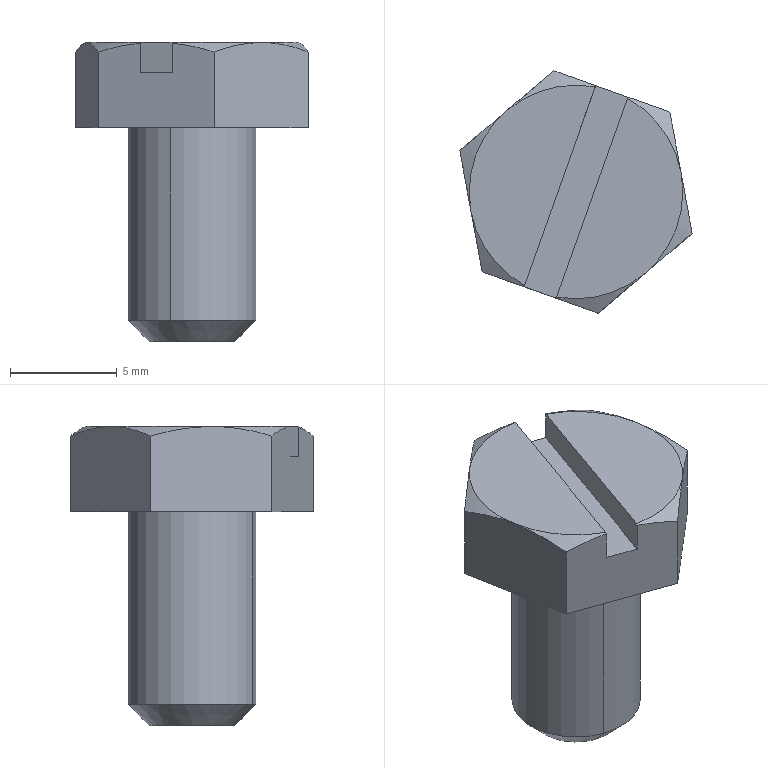Part | SolidWorks | features BaseBody 1 | 1 solid | 23 faces | box 10.878 x 11.357 x 14 mm | volume 597.287 mm3 | plane 13 | cone 8 | cylinder 2 | commonest cylinder face diameters 6 x2
STEP:
#1=CARTESIAN_POINT('',(398.719,157.843,50.8));
#2=VERTEX_POINT('',#1);
#3=CARTESIAN_POINT('',(400.061,161.611,50.8));
#4=VERTEX_POINT('',#3);
#5=CARTESIAN_POINT('',(399.39,159.727,50.8));
#6=DIRECTION('',(0.,0.,-1.));
#7=DIRECTION('',(-0.3355,-0.942,0.));
#8=AXIS2_PLACEMENT_3D('',#5,#6,#7);
#9=CIRCLE('',#8,2.);
#10=EDGE_CURVE('',#2,#4,#9,.T.);
#11=ORIENTED_EDGE('',*,*,#10,.F.);
#12=CARTESIAN_POINT('',(398.384,156.9,51.8));
#13=VERTEX_POINT('',#12);
#14=CARTESIAN_POINT('',(398.719,157.843,50.8));
#15=DIRECTION('',(-0.2372,-0.6661,0.7071));
#16=VECTOR('',#15,1000.);
#17=LINE('',#14,#16);
#18=EDGE_CURVE('',#2,#13,#17,.T.);
#19=ORIENTED_EDGE('',*,*,#18,.T.);
#20=CARTESIAN_POINT('',(400.396,162.553,51.8));
#21=VERTEX_POINT('',#20);
#22=CARTESIAN_POINT('',(399.39,159.727,51.8));
#23=DIRECTION('',(0.,0.,1.));
#24=DIRECTION('',(-0.3355,-0.942,0.));
#25=AXIS2_PLACEMENT_3D('',#22,#23,#24);
#26=CIRCLE('',#25,3.);
#27=EDGE_CURVE('',#21,#13,#26,.T.);
#28=ORIENTED_EDGE('',*,*,#27,.F.);
#29=CARTESIAN_POINT('',(400.061,161.611,50.8));
#30=DIRECTION('',(0.2372,0.6661,0.7071));
#31=VECTOR('',#30,1000.);
#32=LINE('',#29,#31);
#33=EDGE_CURVE('',#4,#21,#32,.T.);
#34=ORIENTED_EDGE('',*,*,#33,.F.);
#35=EDGE_LOOP('',(#11,#19,#28,#34));
#36=FACE_OUTER_BOUND('',#35,.T.);
#37=CARTESIAN_POINT('',(399.39,159.727,50.8));
#38=DIRECTION('',(0.,0.,1.));
#39=DIRECTION('',(0.3355,0.942,0.));
#40=AXIS2_PLACEMENT_3D('',#37,#38,#39);
#41=CONICAL_SURFACE('',#40,2.,0.7854);
#42=ADVANCED_FACE('',(#36),#41,.T.);
#43=ORIENTED_EDGE('',*,*,#27,.T.);
#44=CARTESIAN_POINT('',(398.384,156.9,60.8));
#45=VERTEX_POINT('',#44);
#46=CARTESIAN_POINT('',(398.384,156.9,50.8));
#47=DIRECTION('',(0.,0.,1.));
#48=VECTOR('',#47,1000.);
#49=LINE('',#46,#48);
#50=EDGE_CURVE('',#13,#45,#49,.T.);
#51=ORIENTED_EDGE('',*,*,#50,.T.);
#52=CARTESIAN_POINT('',(400.396,162.553,60.8));
#53=VERTEX_POINT('',#52);
#54=CARTESIAN_POINT('',(399.39,159.727,60.8));
#55=DIRECTION('',(0.,0.,-1.));
#56=DIRECTION('',(-0.3355,-0.942,0.));
#57=AXIS2_PLACEMENT_3D('',#54,#55,#56);
#58=CIRCLE('',#57,3.);
#59=EDGE_CURVE('',#45,#53,#58,.T.);
#60=ORIENTED_EDGE('',*,*,#59,.T.);
#61=CARTESIAN_POINT('',(400.396,162.553,50.8));
#62=DIRECTION('',(0.,0.,1.));
#63=VECTOR('',#62,1000.);
#64=LINE('',#61,#63);
#65=EDGE_CURVE('',#21,#53,#64,.T.);
#66=ORIENTED_EDGE('',*,*,#65,.F.);
#67=EDGE_LOOP('',(#43,#51,#60,#66));
#68=FACE_OUTER_BOUND('',#67,.T.);
#69=CARTESIAN_POINT('',(399.39,159.727,50.8));
#70=DIRECTION('',(0.,0.,1.));
#71=DIRECTION('',(0.3355,0.942,0.));
#72=AXIS2_PLACEMENT_3D('',#69,#70,#71);
#73=CYLINDRICAL_SURFACE('',#72,3.);
#74=ADVANCED_FACE('',(#68),#73,.T.);
#75=CARTESIAN_POINT('',(393.951,161.664,60.8));
#76=VERTEX_POINT('',#75);
#77=CARTESIAN_POINT('',(398.348,165.405,60.8));
#78=VERTEX_POINT('',#77);
#79=CARTESIAN_POINT('',(398.348,165.405,60.8));
#80=DIRECTION('',(0.7616,0.6481,0.));
#81=VECTOR('',#80,1000.);
#82=LINE('',#79,#81);
#83=EDGE_CURVE('',#76,#78,#82,.T.);
#84=ORIENTED_EDGE('',*,*,#83,.T.);
#85=CARTESIAN_POINT('',(403.787,163.468,60.8));
#86=VERTEX_POINT('',#85);
#87=CARTESIAN_POINT('',(403.787,163.468,60.8));
#88=DIRECTION('',(0.942,-0.3355,0.));
#89=VECTOR('',#88,1000.);
#90=LINE('',#87,#89);
#91=EDGE_CURVE('',#78,#86,#90,.T.);
#92=ORIENTED_EDGE('',*,*,#91,.T.);
#93=CARTESIAN_POINT('',(404.829,157.79,60.8));
#94=VERTEX_POINT('',#93);
#95=CARTESIAN_POINT('',(403.787,163.468,60.8));
#96=DIRECTION('',(0.1805,-0.9836,0.));
#97=VECTOR('',#96,1000.);
#98=LINE('',#95,#97);
#99=EDGE_CURVE('',#86,#94,#98,.T.);
#100=ORIENTED_EDGE('',*,*,#99,.T.);
#101=CARTESIAN_POINT('',(400.432,154.048,60.8));
#102=VERTEX_POINT('',#101);
#103=CARTESIAN_POINT('',(400.432,154.048,60.8));
#104=DIRECTION('',(-0.7616,-0.6481,0.));
#105=VECTOR('',#104,1000.);
#106=LINE('',#103,#105);
#107=EDGE_CURVE('',#94,#102,#106,.T.);
#108=ORIENTED_EDGE('',*,*,#107,.T.);
#109=CARTESIAN_POINT('',(394.993,155.985,60.8));
#110=VERTEX_POINT('',#109);
#111=CARTESIAN_POINT('',(400.432,154.048,60.8));
#112=DIRECTION('',(-0.942,0.3355,0.));
#113=VECTOR('',#112,1000.);
#114=LINE('',#111,#113);
#115=EDGE_CURVE('',#102,#110,#114,.T.);
#116=ORIENTED_EDGE('',*,*,#115,.T.);
#117=CARTESIAN_POINT('',(394.993,155.985,60.8));
#118=DIRECTION('',(-0.1805,0.9836,0.));
#119=VECTOR('',#118,1000.);
#120=LINE('',#117,#119);
#121=EDGE_CURVE('',#110,#76,#120,.T.);
#122=ORIENTED_EDGE('',*,*,#121,.T.);
#123=EDGE_LOOP('',(#84,#92,#100,#108,#116,#122));
#124=FACE_OUTER_BOUND('',#123,.T.);
#125=CARTESIAN_POINT('',(399.39,159.727,60.8));
#126=DIRECTION('',(0.,0.,-1.));
#127=DIRECTION('',(-0.3355,-0.942,0.));
#128=AXIS2_PLACEMENT_3D('',#125,#126,#127);
#129=CIRCLE('',#128,3.);
#130=EDGE_CURVE('',#53,#45,#129,.T.);
#131=ORIENTED_EDGE('',*,*,#130,.F.);
#132=ORIENTED_EDGE('',*,*,#59,.F.);
#133=EDGE_LOOP('',(#131,#132));
#134=FACE_BOUND('',#133,.T.);
#135=CARTESIAN_POINT('',(398.348,165.405,60.8));
#136=DIRECTION('',(0.,0.,-1.));
#137=DIRECTION('',(-0.3355,-0.942,0.));
#138=AXIS2_PLACEMENT_3D('',#135,#136,#137);
#139=PLANE('',#138);
#140=ADVANCED_FACE('',(#124,#134),#139,.T.);
#141=CARTESIAN_POINT('',(404.308,160.629,64.8));
#142=VERTEX_POINT('',#141);
#143=CARTESIAN_POINT('',(401.799,164.108,64.8));
#144=VERTEX_POINT('',#143);
#145=CARTESIAN_POINT('',(399.39,159.727,64.8));
#146=DIRECTION('',(0.,0.,1.));
#147=DIRECTION('',(0.3355,0.942,0.));
#148=AXIS2_PLACEMENT_3D('',#145,#146,#147);
#149=CIRCLE('',#148,5.);
#150=EDGE_CURVE('',#142,#144,#149,.T.);
#151=ORIENTED_EDGE('',*,*,#150,.T.);
#152=CARTESIAN_POINT('',(398.488,154.809,64.8));
#153=VERTEX_POINT('',#152);
#154=CARTESIAN_POINT('',(398.466,154.748,64.8));
#155=DIRECTION('',(0.3355,0.942,0.));
#156=VECTOR('',#155,1000.);
#157=LINE('',#154,#156);
#158=EDGE_CURVE('',#153,#144,#157,.T.);
#159=ORIENTED_EDGE('',*,*,#158,.F.);
#160=CARTESIAN_POINT('',(402.63,155.919,64.8));
#161=VERTEX_POINT('',#160);
#162=CARTESIAN_POINT('',(399.39,159.727,64.8));
#163=DIRECTION('',(0.,0.,1.));
#164=DIRECTION('',(0.3355,0.942,0.));
#165=AXIS2_PLACEMENT_3D('',#162,#163,#164);
#166=CIRCLE('',#165,5.);
#167=EDGE_CURVE('',#153,#161,#166,.T.);
#168=ORIENTED_EDGE('',*,*,#167,.T.);
#169=CARTESIAN_POINT('',(399.39,159.727,64.8));
#170=DIRECTION('',(0.,0.,1.));
#171=DIRECTION('',(0.3355,0.942,0.));
#172=AXIS2_PLACEMENT_3D('',#169,#170,#171);
#173=CIRCLE('',#172,5.);
#174=EDGE_CURVE('',#161,#142,#173,.T.);
#175=ORIENTED_EDGE('',*,*,#174,.T.);
#176=EDGE_LOOP('',(#151,#159,#168,#175));
#177=FACE_OUTER_BOUND('',#176,.T.);
#178=CARTESIAN_POINT('',(398.348,165.405,64.8));
#179=DIRECTION('',(0.,0.,-1.));
#180=DIRECTION('',(-0.3355,-0.942,0.));
#181=AXIS2_PLACEMENT_3D('',#178,#179,#180);
#182=PLANE('',#181);
#183=ADVANCED_FACE('',(#177),#182,.F.);
#184=CARTESIAN_POINT('',(398.348,165.405,64.353));
#185=VERTEX_POINT('',#184);
#186=CARTESIAN_POINT('',(396.15,163.534,64.8));
#187=VERTEX_POINT('',#186);
#188=CARTESIAN_POINT('',(398.348,165.405,64.353));
#189=CARTESIAN_POINT('',(397.629,164.793,64.626));
#190=CARTESIAN_POINT('',(396.899,164.172,64.8));
#191=CARTESIAN_POINT('',(396.15,163.534,64.8));
#192=B_SPLINE_CURVE_WITH_KNOTS('',3,(#188,#189,#190,#191),.UNSPECIFIED.,.F.,.F.,(4,4),(0.000000238,0.002921),.UNSPECIFIED.);
#193=EDGE_CURVE('',#185,#187,#192,.T.);
#194=ORIENTED_EDGE('',*,*,#193,.F.);
#195=CARTESIAN_POINT('',(398.348,165.405,60.8));
#196=DIRECTION('',(0.,0.,1.));
#197=VECTOR('',#196,1000.);
#198=LINE('',#195,#197);
#199=EDGE_CURVE('',#78,#185,#198,.T.);
#200=ORIENTED_EDGE('',*,*,#199,.F.);
#201=ORIENTED_EDGE('',*,*,#83,.F.);
#202=CARTESIAN_POINT('',(393.951,161.664,64.353));
#203=VERTEX_POINT('',#202);
#204=CARTESIAN_POINT('',(393.951,161.664,60.8));
#205=DIRECTION('',(0.,0.,1.));
#206=VECTOR('',#205,1000.);
#207=LINE('',#204,#206);
#208=EDGE_CURVE('',#76,#203,#207,.T.);
#209=ORIENTED_EDGE('',*,*,#208,.T.);
#210=CARTESIAN_POINT('',(396.15,163.534,64.8));
#211=CARTESIAN_POINT('',(395.963,163.376,64.8));
#212=CARTESIAN_POINT('',(395.776,163.216,64.789));
#213=CARTESIAN_POINT('',(395.405,162.901,64.749));
#214=CARTESIAN_POINT('',(395.221,162.744,64.718));
#215=CARTESIAN_POINT('',(394.672,162.277,64.602));
#216=CARTESIAN_POINT('',(394.31,161.969,64.489));
#217=CARTESIAN_POINT('',(393.951,161.664,64.353));
#218=B_SPLINE_CURVE_WITH_KNOTS('',3,(#210,#211,#212,#213,#214,#215,#216,#217),.UNSPECIFIED.,.F.,.F.,(4,2,2,4),(0.002921,0.003649,0.004376,0.005831),.UNSPECIFIED.);
#219=EDGE_CURVE('',#187,#203,#218,.T.);
#220=ORIENTED_EDGE('',*,*,#219,.F.);
#221=EDGE_LOOP('',(#194,#200,#201,#209,#220));
#222=FACE_OUTER_BOUND('',#221,.T.);
#223=CARTESIAN_POINT('',(398.348,165.405,60.8));
#224=DIRECTION('',(0.6481,-0.7616,0.));
#225=DIRECTION('',(-0.7616,-0.6481,0.));
#226=AXIS2_PLACEMENT_3D('',#223,#224,#225);
#227=PLANE('',#226);
#228=ADVANCED_FACE('',(#222),#227,.F.);
#229=CARTESIAN_POINT('',(403.787,163.468,64.353));
#230=VERTEX_POINT('',#229);
#231=CARTESIAN_POINT('',(401.821,164.168,64.763));
#232=VERTEX_POINT('',#231);
#233=CARTESIAN_POINT('',(403.787,163.468,64.353));
#234=CARTESIAN_POINT('',(403.465,163.583,64.452));
#235=CARTESIAN_POINT('',(403.138,163.699,64.539));
#236=CARTESIAN_POINT('',(402.482,163.933,64.679));
#237=CARTESIAN_POINT('',(402.152,164.05,64.731));
#238=CARTESIAN_POINT('',(401.821,164.168,64.763));
#239=B_SPLINE_CURVE_WITH_KNOTS('',3,(#233,#234,#235,#236,#237,#238),.UNSPECIFIED.,.F.,.F.,(4,2,4),(0.005386,0.006447,0.007508),.UNSPECIFIED.);
#240=EDGE_CURVE('',#230,#232,#239,.T.);
#241=ORIENTED_EDGE('',*,*,#240,.F.);
#242=CARTESIAN_POINT('',(403.787,163.468,60.8));
#243=DIRECTION('',(0.,0.,1.));
#244=VECTOR('',#243,1000.);
#245=LINE('',#242,#244);
#246=EDGE_CURVE('',#86,#230,#245,.T.);
#247=ORIENTED_EDGE('',*,*,#246,.F.);
#248=ORIENTED_EDGE('',*,*,#91,.F.);
#249=ORIENTED_EDGE('',*,*,#199,.T.);
#250=CARTESIAN_POINT('',(400.314,164.705,64.763));
#251=VERTEX_POINT('',#250);
#252=CARTESIAN_POINT('',(400.314,164.705,64.763));
#253=CARTESIAN_POINT('',(399.641,164.945,64.698));
#254=CARTESIAN_POINT('',(398.989,165.177,64.55));
#255=CARTESIAN_POINT('',(398.348,165.405,64.353));
#256=B_SPLINE_CURVE_WITH_KNOTS('',3,(#252,#253,#254,#255),.UNSPECIFIED.,.F.,.F.,(4,4),(0.009104,0.01123),.UNSPECIFIED.);
#257=EDGE_CURVE('',#251,#185,#256,.T.);
#258=ORIENTED_EDGE('',*,*,#257,.F.);
#259=CARTESIAN_POINT('',(400.314,164.705,63.4));
#260=VERTEX_POINT('',#259);
#261=CARTESIAN_POINT('',(400.314,164.705,63.4));
#262=DIRECTION('',(0.,0.,1.));
#263=VECTOR('',#262,1000.);
#264=LINE('',#261,#263);
#265=EDGE_CURVE('',#260,#251,#264,.T.);
#266=ORIENTED_EDGE('',*,*,#265,.F.);
#267=CARTESIAN_POINT('',(401.821,164.168,63.4));
#268=VERTEX_POINT('',#267);
#269=CARTESIAN_POINT('',(400.314,164.705,63.4));
#270=DIRECTION('',(-0.942,0.3355,0.));
#271=VECTOR('',#270,1000.);
#272=LINE('',#269,#271);
#273=EDGE_CURVE('',#268,#260,#272,.T.);
#274=ORIENTED_EDGE('',*,*,#273,.F.);
#275=CARTESIAN_POINT('',(401.821,164.168,63.4));
#276=DIRECTION('',(0.,0.,1.));
#277=VECTOR('',#276,1000.);
#278=LINE('',#275,#277);
#279=EDGE_CURVE('',#268,#232,#278,.T.);
#280=ORIENTED_EDGE('',*,*,#279,.T.);
#281=EDGE_LOOP('',(#241,#247,#248,#249,#258,#266,#274,#280));
#282=FACE_OUTER_BOUND('',#281,.T.);
#283=CARTESIAN_POINT('',(403.787,163.468,60.8));
#284=DIRECTION('',(-0.3355,-0.942,0.));
#285=DIRECTION('',(-0.942,0.3355,0.));
#286=AXIS2_PLACEMENT_3D('',#283,#284,#285);
#287=PLANE('',#286);
#288=ADVANCED_FACE('',(#282),#287,.F.);
#289=CARTESIAN_POINT('',(404.829,157.79,64.353));
#290=VERTEX_POINT('',#289);
#291=CARTESIAN_POINT('',(404.829,157.79,64.353));
#292=CARTESIAN_POINT('',(404.658,158.719,64.626));
#293=CARTESIAN_POINT('',(404.485,159.662,64.8));
#294=CARTESIAN_POINT('',(404.308,160.629,64.8));
#295=B_SPLINE_CURVE_WITH_KNOTS('',3,(#291,#292,#293,#294),.UNSPECIFIED.,.F.,.F.,(4,4),(0.000000238,0.002921),.UNSPECIFIED.);
#296=EDGE_CURVE('',#290,#142,#295,.T.);
#297=ORIENTED_EDGE('',*,*,#296,.F.);
#298=CARTESIAN_POINT('',(404.829,157.79,60.8));
#299=DIRECTION('',(0.,0.,1.));
#300=VECTOR('',#299,1000.);
#301=LINE('',#298,#300);
#302=EDGE_CURVE('',#94,#290,#301,.T.);
#303=ORIENTED_EDGE('',*,*,#302,.F.);
#304=ORIENTED_EDGE('',*,*,#99,.F.);
#305=ORIENTED_EDGE('',*,*,#246,.T.);
#306=CARTESIAN_POINT('',(404.308,160.629,64.8));
#307=CARTESIAN_POINT('',(404.264,160.87,64.8));
#308=CARTESIAN_POINT('',(404.219,161.112,64.789));
#309=CARTESIAN_POINT('',(404.131,161.591,64.749));
#310=CARTESIAN_POINT('',(404.088,161.829,64.718));
#311=CARTESIAN_POINT('',(403.958,162.538,64.602));
#312=CARTESIAN_POINT('',(403.872,163.005,64.489));
#313=CARTESIAN_POINT('',(403.787,163.468,64.353));
#314=B_SPLINE_CURVE_WITH_KNOTS('',3,(#306,#307,#308,#309,#310,#311,#312,#313),.UNSPECIFIED.,.F.,.F.,(4,2,2,4),(0.002921,0.003649,0.004376,0.005831),.UNSPECIFIED.);
#315=EDGE_CURVE('',#142,#230,#314,.T.);
#316=ORIENTED_EDGE('',*,*,#315,.F.);
#317=EDGE_LOOP('',(#297,#303,#304,#305,#316));
#318=FACE_OUTER_BOUND('',#317,.T.);
#319=CARTESIAN_POINT('',(403.787,163.468,60.8));
#320=DIRECTION('',(-0.9836,-0.1805,0.));
#321=DIRECTION('',(-0.1805,0.9836,0.));
#322=AXIS2_PLACEMENT_3D('',#319,#320,#321);
#323=PLANE('',#322);
#324=ADVANCED_FACE('',(#318),#323,.F.);
#325=CARTESIAN_POINT('',(400.432,154.048,64.353));
#326=VERTEX_POINT('',#325);
#327=CARTESIAN_POINT('',(400.432,154.048,64.353));
#328=CARTESIAN_POINT('',(401.151,154.66,64.626));
#329=CARTESIAN_POINT('',(401.881,155.281,64.8));
#330=CARTESIAN_POINT('',(402.63,155.919,64.8));
#331=B_SPLINE_CURVE_WITH_KNOTS('',3,(#327,#328,#329,#330),.UNSPECIFIED.,.F.,.F.,(4,4),(0.000000238,0.002921),.UNSPECIFIED.);
#332=EDGE_CURVE('',#326,#161,#331,.T.);
#333=ORIENTED_EDGE('',*,*,#332,.F.);
#334=CARTESIAN_POINT('',(400.432,154.048,60.8));
#335=DIRECTION('',(0.,0.,1.));
#336=VECTOR('',#335,1000.);
#337=LINE('',#334,#336);
#338=EDGE_CURVE('',#102,#326,#337,.T.);
#339=ORIENTED_EDGE('',*,*,#338,.F.);
#340=ORIENTED_EDGE('',*,*,#107,.F.);
#341=ORIENTED_EDGE('',*,*,#302,.T.);
#342=CARTESIAN_POINT('',(402.63,155.919,64.8));
#343=CARTESIAN_POINT('',(402.817,156.078,64.8));
#344=CARTESIAN_POINT('',(403.004,156.237,64.789));
#345=CARTESIAN_POINT('',(403.375,156.553,64.749));
#346=CARTESIAN_POINT('',(403.559,156.709,64.718));
#347=CARTESIAN_POINT('',(404.108,157.177,64.602));
#348=CARTESIAN_POINT('',(404.47,157.484,64.489));
#349=CARTESIAN_POINT('',(404.829,157.79,64.353));
#350=B_SPLINE_CURVE_WITH_KNOTS('',3,(#342,#343,#344,#345,#346,#347,#348,#349),.UNSPECIFIED.,.F.,.F.,(4,2,2,4),(0.002921,0.003649,0.004376,0.005831),.UNSPECIFIED.);
#351=EDGE_CURVE('',#161,#290,#350,.T.);
#352=ORIENTED_EDGE('',*,*,#351,.F.);
#353=EDGE_LOOP('',(#333,#339,#340,#341,#352));
#354=FACE_OUTER_BOUND('',#353,.T.);
#355=CARTESIAN_POINT('',(400.432,154.048,60.8));
#356=DIRECTION('',(-0.6481,0.7616,0.));
#357=DIRECTION('',(0.7616,0.6481,0.));
#358=AXIS2_PLACEMENT_3D('',#355,#356,#357);
#359=PLANE('',#358);
#360=ADVANCED_FACE('',(#354),#359,.F.);
#361=CARTESIAN_POINT('',(394.993,155.985,64.353));
#362=VERTEX_POINT('',#361);
#363=CARTESIAN_POINT('',(396.959,155.285,64.763));
#364=VERTEX_POINT('',#363);
#365=CARTESIAN_POINT('',(394.993,155.985,64.353));
#366=CARTESIAN_POINT('',(395.634,155.757,64.55));
#367=CARTESIAN_POINT('',(396.286,155.524,64.698));
#368=CARTESIAN_POINT('',(396.959,155.285,64.763));
#369=B_SPLINE_CURVE_WITH_KNOTS('',3,(#365,#366,#367,#368),.UNSPECIFIED.,.F.,.F.,(4,4),(0.0154,0.01752),.UNSPECIFIED.);
#370=EDGE_CURVE('',#362,#364,#369,.T.);
#371=ORIENTED_EDGE('',*,*,#370,.F.);
#372=CARTESIAN_POINT('',(394.993,155.985,60.8));
#373=DIRECTION('',(0.,0.,1.));
#374=VECTOR('',#373,1000.);
#375=LINE('',#372,#374);
#376=EDGE_CURVE('',#110,#362,#375,.T.);
#377=ORIENTED_EDGE('',*,*,#376,.F.);
#378=ORIENTED_EDGE('',*,*,#115,.F.);
#379=ORIENTED_EDGE('',*,*,#338,.T.);
#380=CARTESIAN_POINT('',(398.466,154.748,64.763));
#381=VERTEX_POINT('',#380);
#382=CARTESIAN_POINT('',(398.466,154.748,64.763));
#383=CARTESIAN_POINT('',(398.798,154.63,64.731));
#384=CARTESIAN_POINT('',(399.127,154.513,64.679));
#385=CARTESIAN_POINT('',(399.783,154.279,64.539));
#386=CARTESIAN_POINT('',(400.11,154.162,64.452));
#387=CARTESIAN_POINT('',(400.432,154.048,64.353));
#388=B_SPLINE_CURVE_WITH_KNOTS('',3,(#382,#383,#384,#385,#386,#387),.UNSPECIFIED.,.F.,.F.,(4,2,4),(0.01912,0.02018,0.02124),.UNSPECIFIED.);
#389=EDGE_CURVE('',#381,#326,#388,.T.);
#390=ORIENTED_EDGE('',*,*,#389,.F.);
#391=CARTESIAN_POINT('',(398.466,154.748,63.4));
#392=VERTEX_POINT('',#391);
#393=CARTESIAN_POINT('',(398.466,154.748,63.4));
#394=DIRECTION('',(0.,0.,1.));
#395=VECTOR('',#394,1000.);
#396=LINE('',#393,#395);
#397=EDGE_CURVE('',#392,#381,#396,.T.);
#398=ORIENTED_EDGE('',*,*,#397,.F.);
#399=CARTESIAN_POINT('',(396.959,155.285,63.4));
#400=VERTEX_POINT('',#399);
#401=CARTESIAN_POINT('',(398.466,154.748,63.4));
#402=DIRECTION('',(0.942,-0.3355,0.));
#403=VECTOR('',#402,1000.);
#404=LINE('',#401,#403);
#405=EDGE_CURVE('',#400,#392,#404,.T.);
#406=ORIENTED_EDGE('',*,*,#405,.F.);
#407=CARTESIAN_POINT('',(396.959,155.285,63.4));
#408=DIRECTION('',(0.,0.,1.));
#409=VECTOR('',#408,1000.);
#410=LINE('',#407,#409);
#411=EDGE_CURVE('',#400,#364,#410,.T.);
#412=ORIENTED_EDGE('',*,*,#411,.T.);
#413=EDGE_LOOP('',(#371,#377,#378,#379,#390,#398,#406,#412));
#414=FACE_OUTER_BOUND('',#413,.T.);
#415=CARTESIAN_POINT('',(400.432,154.048,60.8));
#416=DIRECTION('',(0.3355,0.942,0.));
#417=DIRECTION('',(0.,0.,-1.));
#418=AXIS2_PLACEMENT_3D('',#415,#416,#417);
#419=PLANE('',#418);
#420=ADVANCED_FACE('',(#414),#419,.F.);
#421=CARTESIAN_POINT('',(394.472,158.824,64.8));
#422=VERTEX_POINT('',#421);
#423=CARTESIAN_POINT('',(393.951,161.664,64.353));
#424=CARTESIAN_POINT('',(394.122,160.735,64.626));
#425=CARTESIAN_POINT('',(394.295,159.792,64.8));
#426=CARTESIAN_POINT('',(394.472,158.824,64.8));
#427=B_SPLINE_CURVE_WITH_KNOTS('',3,(#423,#424,#425,#426),.UNSPECIFIED.,.F.,.F.,(4,4),(0.000000238,0.002921),.UNSPECIFIED.);
#428=EDGE_CURVE('',#203,#422,#427,.T.);
#429=ORIENTED_EDGE('',*,*,#428,.F.);
#430=ORIENTED_EDGE('',*,*,#208,.F.);
#431=ORIENTED_EDGE('',*,*,#121,.F.);
#432=ORIENTED_EDGE('',*,*,#376,.T.);
#433=CARTESIAN_POINT('',(394.472,158.824,64.8));
#434=CARTESIAN_POINT('',(394.516,158.583,64.8));
#435=CARTESIAN_POINT('',(394.561,158.341,64.789));
#436=CARTESIAN_POINT('',(394.649,157.862,64.749));
#437=CARTESIAN_POINT('',(394.692,157.625,64.718));
#438=CARTESIAN_POINT('',(394.822,156.915,64.602));
#439=CARTESIAN_POINT('',(394.908,156.448,64.489));
#440=CARTESIAN_POINT('',(394.993,155.985,64.353));
#441=B_SPLINE_CURVE_WITH_KNOTS('',3,(#433,#434,#435,#436,#437,#438,#439,#440),.UNSPECIFIED.,.F.,.F.,(4,2,2,4),(0.002921,0.003649,0.004376,0.005831),.UNSPECIFIED.);
#442=EDGE_CURVE('',#422,#362,#441,.T.);
#443=ORIENTED_EDGE('',*,*,#442,.F.);
#444=EDGE_LOOP('',(#429,#430,#431,#432,#443));
#445=FACE_OUTER_BOUND('',#444,.T.);
#446=CARTESIAN_POINT('',(394.993,155.985,60.8));
#447=DIRECTION('',(0.9836,0.1805,0.));
#448=DIRECTION('',(0.1805,-0.9836,0.));
#449=AXIS2_PLACEMENT_3D('',#446,#447,#448);
#450=PLANE('',#449);
#451=ADVANCED_FACE('',(#445),#450,.F.);
#452=CARTESIAN_POINT('',(396.981,155.345,64.8));
#453=VERTEX_POINT('',#452);
#454=CARTESIAN_POINT('',(399.39,159.727,64.8));
#455=DIRECTION('',(0.,0.,1.));
#456=DIRECTION('',(0.3355,0.942,0.));
#457=AXIS2_PLACEMENT_3D('',#454,#455,#456);
#458=CIRCLE('',#457,5.);
#459=EDGE_CURVE('',#422,#453,#458,.T.);
#460=ORIENTED_EDGE('',*,*,#459,.T.);
#461=CARTESIAN_POINT('',(400.292,164.645,64.8));
#462=VERTEX_POINT('',#461);
#463=CARTESIAN_POINT('',(396.959,155.285,64.8));
#464=DIRECTION('',(-0.3355,-0.942,0.));
#465=VECTOR('',#464,1000.);
#466=LINE('',#463,#465);
#467=EDGE_CURVE('',#462,#453,#466,.T.);
#468=ORIENTED_EDGE('',*,*,#467,.F.);
#469=CARTESIAN_POINT('',(399.39,159.727,64.8));
#470=DIRECTION('',(0.,0.,1.));
#471=DIRECTION('',(0.3355,0.942,0.));
#472=AXIS2_PLACEMENT_3D('',#469,#470,#471);
#473=CIRCLE('',#472,5.);
#474=EDGE_CURVE('',#462,#187,#473,.T.);
#475=ORIENTED_EDGE('',*,*,#474,.T.);
#476=CARTESIAN_POINT('',(399.39,159.727,64.8));
#477=DIRECTION('',(0.,0.,1.));
#478=DIRECTION('',(0.3355,0.942,0.));
#479=AXIS2_PLACEMENT_3D('',#476,#477,#478);
#480=CIRCLE('',#479,5.);
#481=EDGE_CURVE('',#187,#422,#480,.T.);
#482=ORIENTED_EDGE('',*,*,#481,.T.);
#483=EDGE_LOOP('',(#460,#468,#475,#482));
#484=FACE_OUTER_BOUND('',#483,.T.);
#485=CARTESIAN_POINT('',(398.348,165.405,64.8));
#486=DIRECTION('',(0.,0.,-1.));
#487=DIRECTION('',(-0.3355,-0.942,0.));
#488=AXIS2_PLACEMENT_3D('',#485,#486,#487);
#489=PLANE('',#488);
#490=ADVANCED_FACE('',(#484),#489,.F.);
#491=CARTESIAN_POINT('',(401.821,164.168,64.763));
#492=CARTESIAN_POINT('',(401.814,164.148,64.776));
#493=CARTESIAN_POINT('',(401.807,164.128,64.788));
#494=CARTESIAN_POINT('',(401.799,164.108,64.8));
#495=B_SPLINE_CURVE_WITH_KNOTS('',3,(#491,#492,#493,#494),.UNSPECIFIED.,.F.,.F.,(4,4),(0.006986,0.00706),.UNSPECIFIED.);
#496=EDGE_CURVE('',#232,#144,#495,.T.);
#497=ORIENTED_EDGE('',*,*,#496,.F.);
#498=ORIENTED_EDGE('',*,*,#279,.F.);
#499=CARTESIAN_POINT('',(398.466,154.748,63.4));
#500=DIRECTION('',(0.3355,0.942,0.));
#501=VECTOR('',#500,1000.);
#502=LINE('',#499,#501);
#503=EDGE_CURVE('',#392,#268,#502,.T.);
#504=ORIENTED_EDGE('',*,*,#503,.F.);
#505=ORIENTED_EDGE('',*,*,#397,.T.);
#506=CARTESIAN_POINT('',(398.488,154.809,64.8));
#507=CARTESIAN_POINT('',(398.481,154.788,64.788));
#508=CARTESIAN_POINT('',(398.473,154.768,64.776));
#509=CARTESIAN_POINT('',(398.466,154.748,64.763));
#510=B_SPLINE_CURVE_WITH_KNOTS('',3,(#506,#507,#508,#509),.UNSPECIFIED.,.F.,.F.,(4,4),(0.01814,0.01822),.UNSPECIFIED.);
#511=EDGE_CURVE('',#153,#381,#510,.T.);
#512=ORIENTED_EDGE('',*,*,#511,.F.);
#513=ORIENTED_EDGE('',*,*,#158,.T.);
#514=EDGE_LOOP('',(#497,#498,#504,#505,#512,#513));
#515=FACE_OUTER_BOUND('',#514,.T.);
#516=CARTESIAN_POINT('',(398.466,154.748,63.4));
#517=DIRECTION('',(0.942,-0.3355,0.));
#518=DIRECTION('',(0.,0.,1.));
#519=AXIS2_PLACEMENT_3D('',#516,#517,#518);
#520=PLANE('',#519);
#521=ADVANCED_FACE('',(#515),#520,.F.);
#522=CARTESIAN_POINT('',(396.959,155.285,64.763));
#523=CARTESIAN_POINT('',(396.966,155.305,64.776));
#524=CARTESIAN_POINT('',(396.973,155.325,64.788));
#525=CARTESIAN_POINT('',(396.981,155.345,64.8));
#526=B_SPLINE_CURVE_WITH_KNOTS('',3,(#522,#523,#524,#525),.UNSPECIFIED.,.F.,.F.,(4,4),(0.006986,0.00706),.UNSPECIFIED.);
#527=EDGE_CURVE('',#364,#453,#526,.T.);
#528=ORIENTED_EDGE('',*,*,#527,.F.);
#529=ORIENTED_EDGE('',*,*,#411,.F.);
#530=CARTESIAN_POINT('',(396.959,155.285,63.4));
#531=DIRECTION('',(-0.3355,-0.942,0.));
#532=VECTOR('',#531,1000.);
#533=LINE('',#530,#532);
#534=EDGE_CURVE('',#260,#400,#533,.T.);
#535=ORIENTED_EDGE('',*,*,#534,.F.);
#536=ORIENTED_EDGE('',*,*,#265,.T.);
#537=CARTESIAN_POINT('',(400.292,164.645,64.8));
#538=CARTESIAN_POINT('',(400.299,164.665,64.788));
#539=CARTESIAN_POINT('',(400.307,164.685,64.776));
#540=CARTESIAN_POINT('',(400.314,164.705,64.763));
#541=B_SPLINE_CURVE_WITH_KNOTS('',3,(#537,#538,#539,#540),.UNSPECIFIED.,.F.,.F.,(4,4),(0.01814,0.01822),.UNSPECIFIED.);
#542=EDGE_CURVE('',#462,#251,#541,.T.);
#543=ORIENTED_EDGE('',*,*,#542,.F.);
#544=ORIENTED_EDGE('',*,*,#467,.T.);
#545=EDGE_LOOP('',(#528,#529,#535,#536,#543,#544));
#546=FACE_OUTER_BOUND('',#545,.T.);
#547=CARTESIAN_POINT('',(396.959,155.285,63.4));
#548=DIRECTION('',(-0.942,0.3355,0.));
#549=DIRECTION('',(0.,0.,-1.));
#550=AXIS2_PLACEMENT_3D('',#547,#548,#549);
#551=PLANE('',#550);
#552=ADVANCED_FACE('',(#546),#551,.F.);
#553=ORIENTED_EDGE('',*,*,#273,.T.);
#554=ORIENTED_EDGE('',*,*,#534,.T.);
#555=ORIENTED_EDGE('',*,*,#405,.T.);
#556=ORIENTED_EDGE('',*,*,#503,.T.);
#557=EDGE_LOOP('',(#553,#554,#555,#556));
#558=FACE_OUTER_BOUND('',#557,.T.);
#559=CARTESIAN_POINT('',(401.821,164.168,63.4));
#560=DIRECTION('',(0.,0.,1.));
#561=DIRECTION('',(0.3355,0.942,0.));
#562=AXIS2_PLACEMENT_3D('',#559,#560,#561);
#563=PLANE('',#562);
#564=ADVANCED_FACE('',(#558),#563,.T.);
#565=ORIENTED_EDGE('',*,*,#193,.T.);
#566=ORIENTED_EDGE('',*,*,#474,.F.);
#567=ORIENTED_EDGE('',*,*,#542,.T.);
#568=ORIENTED_EDGE('',*,*,#257,.T.);
#569=EDGE_LOOP('',(#565,#566,#567,#568));
#570=FACE_OUTER_BOUND('',#569,.T.);
#571=CARTESIAN_POINT('',(399.39,159.727,64.8));
#572=DIRECTION('',(0.,0.,-1.));
#573=DIRECTION('',(0.3355,0.942,0.));
#574=AXIS2_PLACEMENT_3D('',#571,#572,#573);
#575=CONICAL_SURFACE('',#574,5.,1.047);
#576=ADVANCED_FACE('',(#570),#575,.T.);
#577=ORIENTED_EDGE('',*,*,#527,.T.);
#578=ORIENTED_EDGE('',*,*,#459,.F.);
#579=ORIENTED_EDGE('',*,*,#442,.T.);
#580=ORIENTED_EDGE('',*,*,#370,.T.);
#581=EDGE_LOOP('',(#577,#578,#579,#580));
#582=FACE_OUTER_BOUND('',#581,.T.);
#583=CARTESIAN_POINT('',(399.39,159.727,64.8));
#584=DIRECTION('',(0.,0.,-1.));
#585=DIRECTION('',(0.3355,0.942,0.));
#586=AXIS2_PLACEMENT_3D('',#583,#584,#585);
#587=CONICAL_SURFACE('',#586,5.,1.047);
#588=ADVANCED_FACE('',(#582),#587,.T.);
#589=ORIENTED_EDGE('',*,*,#332,.T.);
#590=ORIENTED_EDGE('',*,*,#167,.F.);
#591=ORIENTED_EDGE('',*,*,#511,.T.);
#592=ORIENTED_EDGE('',*,*,#389,.T.);
#593=EDGE_LOOP('',(#589,#590,#591,#592));
#594=FACE_OUTER_BOUND('',#593,.T.);
#595=CARTESIAN_POINT('',(399.39,159.727,64.8));
#596=DIRECTION('',(0.,0.,-1.));
#597=DIRECTION('',(0.3355,0.942,0.));
#598=AXIS2_PLACEMENT_3D('',#595,#596,#597);
#599=CONICAL_SURFACE('',#598,5.,1.047);
#600=ADVANCED_FACE('',(#594),#599,.T.);
#601=ORIENTED_EDGE('',*,*,#496,.T.);
#602=ORIENTED_EDGE('',*,*,#150,.F.);
#603=ORIENTED_EDGE('',*,*,#315,.T.);
#604=ORIENTED_EDGE('',*,*,#240,.T.);
#605=EDGE_LOOP('',(#601,#602,#603,#604));
#606=FACE_OUTER_BOUND('',#605,.T.);
#607=CARTESIAN_POINT('',(399.39,159.727,64.8));
#608=DIRECTION('',(0.,0.,-1.));
#609=DIRECTION('',(0.3355,0.942,0.));
#610=AXIS2_PLACEMENT_3D('',#607,#608,#609);
#611=CONICAL_SURFACE('',#610,5.,1.047);
#612=ADVANCED_FACE('',(#606),#611,.T.);
#613=ORIENTED_EDGE('',*,*,#428,.T.);
#614=ORIENTED_EDGE('',*,*,#481,.F.);
#615=ORIENTED_EDGE('',*,*,#219,.T.);
#616=EDGE_LOOP('',(#613,#614,#615));
#617=FACE_OUTER_BOUND('',#616,.T.);
#618=CARTESIAN_POINT('',(399.39,159.727,64.8));
#619=DIRECTION('',(0.,0.,-1.));
#620=DIRECTION('',(0.3355,0.942,0.));
#621=AXIS2_PLACEMENT_3D('',#618,#619,#620);
#622=CONICAL_SURFACE('',#621,5.,1.047);
#623=ADVANCED_FACE('',(#617),#622,.T.);
#624=ORIENTED_EDGE('',*,*,#296,.T.);
#625=ORIENTED_EDGE('',*,*,#174,.F.);
#626=ORIENTED_EDGE('',*,*,#351,.T.);
#627=EDGE_LOOP('',(#624,#625,#626));
#628=FACE_OUTER_BOUND('',#627,.T.);
#629=CARTESIAN_POINT('',(399.39,159.727,64.8));
#630=DIRECTION('',(0.,0.,-1.));
#631=DIRECTION('',(0.3355,0.942,0.));
#632=AXIS2_PLACEMENT_3D('',#629,#630,#631);
#633=CONICAL_SURFACE('',#632,5.,1.047);
#634=ADVANCED_FACE('',(#628),#633,.T.);
#635=ORIENTED_EDGE('',*,*,#50,.F.);
#636=CARTESIAN_POINT('',(399.39,159.727,51.8));
#637=DIRECTION('',(0.,0.,1.));
#638=DIRECTION('',(-0.3355,-0.942,0.));
#639=AXIS2_PLACEMENT_3D('',#636,#637,#638);
#640=CIRCLE('',#639,3.);
#641=EDGE_CURVE('',#13,#21,#640,.T.);
#642=ORIENTED_EDGE('',*,*,#641,.T.);
#643=ORIENTED_EDGE('',*,*,#65,.T.);
#644=ORIENTED_EDGE('',*,*,#130,.T.);
#645=EDGE_LOOP('',(#635,#642,#643,#644));
#646=FACE_OUTER_BOUND('',#645,.T.);
#647=CARTESIAN_POINT('',(399.39,159.727,50.8));
#648=DIRECTION('',(0.,0.,1.));
#649=DIRECTION('',(0.3355,0.942,0.));
#650=AXIS2_PLACEMENT_3D('',#647,#648,#649);
#651=CYLINDRICAL_SURFACE('',#650,3.);
#652=ADVANCED_FACE('',(#646),#651,.T.);
#653=CARTESIAN_POINT('',(399.39,159.727,50.8));
#654=DIRECTION('',(0.,0.,-1.));
#655=DIRECTION('',(-0.3355,-0.942,0.));
#656=AXIS2_PLACEMENT_3D('',#653,#654,#655);
#657=CIRCLE('',#656,2.);
#658=EDGE_CURVE('',#4,#2,#657,.T.);
#659=ORIENTED_EDGE('',*,*,#658,.T.);
#660=ORIENTED_EDGE('',*,*,#10,.T.);
#661=EDGE_LOOP('',(#659,#660));
#662=FACE_OUTER_BOUND('',#661,.T.);
#663=CARTESIAN_POINT('',(399.39,159.727,50.8));
#664=DIRECTION('',(0.,0.,-1.));
#665=DIRECTION('',(-0.3355,-0.942,0.));
#666=AXIS2_PLACEMENT_3D('',#663,#664,#665);
#667=PLANE('',#666);
#668=ADVANCED_FACE('',(#662),#667,.T.);
#669=ORIENTED_EDGE('',*,*,#18,.F.);
#670=ORIENTED_EDGE('',*,*,#658,.F.);
#671=ORIENTED_EDGE('',*,*,#33,.T.);
#672=ORIENTED_EDGE('',*,*,#641,.F.);
#673=EDGE_LOOP('',(#669,#670,#671,#672));
#674=FACE_OUTER_BOUND('',#673,.T.);
#675=CARTESIAN_POINT('',(399.39,159.727,50.8));
#676=DIRECTION('',(0.,0.,1.));
#677=DIRECTION('',(0.3355,0.942,0.));
#678=AXIS2_PLACEMENT_3D('',#675,#676,#677);
#679=CONICAL_SURFACE('',#678,2.,0.7854);
#680=ADVANCED_FACE('',(#674),#679,.T.);
#681=CLOSED_SHELL('',(#42,#74,#140,#183,#228,#288,#324,#360,#420,#451,#490,#521,#552,#564,#576,#588,#600,#612,#623,#634,#652,#668,#680));
#682=MANIFOLD_SOLID_BREP('',#681);
#683=CARTESIAN_POINT('',(0.,0.,0.));
#684=DIRECTION('',(0.,0.,1.));
#685=DIRECTION('',(1.,0.,0.));
#686=AXIS2_PLACEMENT_3D('',#683,#684,#685);
#687=(LENGTH_UNIT()NAMED_UNIT(*)SI_UNIT(.MILLI.,.METRE.));
#688=UNCERTAINTY_MEASURE_WITH_UNIT(LENGTH_MEASURE(0.00001),#687,'','');
#689=(NAMED_UNIT(*)PLANE_ANGLE_UNIT()SI_UNIT($,.RADIAN.));
#690=(NAMED_UNIT(*)SI_UNIT($,.STERADIAN.)SOLID_ANGLE_UNIT());
#691=(GEOMETRIC_REPRESENTATION_CONTEXT(3)GLOBAL_UNCERTAINTY_ASSIGNED_CONTEXT((#688))GLOBAL_UNIT_ASSIGNED_CONTEXT((#687,#689,#690))REPRESENTATION_CONTEXT('',''));
#692=ADVANCED_BREP_SHAPE_REPRESENTATION('',(#682,#686),#691);